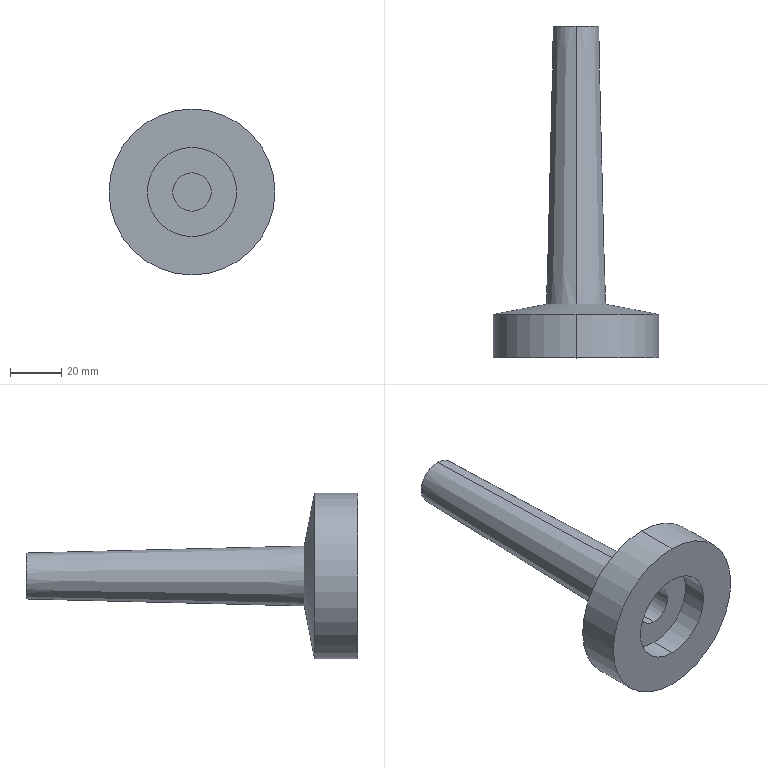Part | SolidWorks | features ICE 2, Revolution 1 | 1 solid | 14 faces | box 65 x 130 x 65 mm | volume 88701 mm3 | cylinder 6 | cone 4 | plane 4 | commonest cylinder face diameters 15 x2 35 x2 65 x2
STEP:
#1=CARTESIAN_POINT('',(0.,20.,7.5));
#2=VERTEX_POINT('',#1);
#3=CARTESIAN_POINT('',(0.,20.,-7.5));
#4=VERTEX_POINT('',#3);
#5=CARTESIAN_POINT('',(0.,20.,0.));
#6=DIRECTION('',(0.,-1.,0.));
#7=DIRECTION('',(0.,0.,-1.));
#8=AXIS2_PLACEMENT_3D('',#5,#6,#7);
#9=CIRCLE('',#8,7.5);
#10=EDGE_CURVE('',#2,#4,#9,.T.);
#11=ORIENTED_EDGE('',*,*,#10,.F.);
#12=CARTESIAN_POINT('',(0.,10.,7.5));
#13=VERTEX_POINT('',#12);
#14=CARTESIAN_POINT('',(0.,20.,7.5));
#15=DIRECTION('',(0.,-1.,0.));
#16=VECTOR('',#15,1000.);
#17=LINE('',#14,#16);
#18=EDGE_CURVE('',#2,#13,#17,.T.);
#19=ORIENTED_EDGE('',*,*,#18,.T.);
#20=CARTESIAN_POINT('',(0.,10.,-7.5));
#21=VERTEX_POINT('',#20);
#22=CARTESIAN_POINT('',(0.,10.,0.));
#23=DIRECTION('',(0.,-1.,0.));
#24=DIRECTION('',(0.,0.,-1.));
#25=AXIS2_PLACEMENT_3D('',#22,#23,#24);
#26=CIRCLE('',#25,7.5);
#27=EDGE_CURVE('',#13,#21,#26,.T.);
#28=ORIENTED_EDGE('',*,*,#27,.T.);
#29=CARTESIAN_POINT('',(0.,20.,-7.5));
#30=DIRECTION('',(0.,-1.,0.));
#31=VECTOR('',#30,1000.);
#32=LINE('',#29,#31);
#33=EDGE_CURVE('',#4,#21,#32,.T.);
#34=ORIENTED_EDGE('',*,*,#33,.F.);
#35=EDGE_LOOP('',(#11,#19,#28,#34));
#36=FACE_OUTER_BOUND('',#35,.T.);
#37=CARTESIAN_POINT('',(0.,20.,0.));
#38=DIRECTION('',(0.,-1.,0.));
#39=DIRECTION('',(0.,0.,-1.));
#40=AXIS2_PLACEMENT_3D('',#37,#38,#39);
#41=CYLINDRICAL_SURFACE('',#40,7.5);
#42=ADVANCED_FACE('',(#36),#41,.F.);
#43=CARTESIAN_POINT('',(0.,10.,17.5));
#44=VERTEX_POINT('',#43);
#45=CARTESIAN_POINT('',(0.,10.,-17.5));
#46=VERTEX_POINT('',#45);
#47=CARTESIAN_POINT('',(0.,10.,0.));
#48=DIRECTION('',(0.,-1.,0.));
#49=DIRECTION('',(0.,0.,-1.));
#50=AXIS2_PLACEMENT_3D('',#47,#48,#49);
#51=CIRCLE('',#50,17.5);
#52=EDGE_CURVE('',#44,#46,#51,.T.);
#53=ORIENTED_EDGE('',*,*,#52,.F.);
#54=CARTESIAN_POINT('',(0.,0.,17.5));
#55=VERTEX_POINT('',#54);
#56=CARTESIAN_POINT('',(0.,10.,17.5));
#57=DIRECTION('',(0.,-1.,0.));
#58=VECTOR('',#57,1000.);
#59=LINE('',#56,#58);
#60=EDGE_CURVE('',#44,#55,#59,.T.);
#61=ORIENTED_EDGE('',*,*,#60,.T.);
#62=CARTESIAN_POINT('',(0.,0.,-17.5));
#63=VERTEX_POINT('',#62);
#64=CARTESIAN_POINT('',(0.,0.,0.));
#65=DIRECTION('',(0.,-1.,0.));
#66=DIRECTION('',(0.,0.,-1.));
#67=AXIS2_PLACEMENT_3D('',#64,#65,#66);
#68=CIRCLE('',#67,17.5);
#69=EDGE_CURVE('',#55,#63,#68,.T.);
#70=ORIENTED_EDGE('',*,*,#69,.T.);
#71=CARTESIAN_POINT('',(0.,10.,-17.5));
#72=DIRECTION('',(0.,-1.,0.));
#73=VECTOR('',#72,1000.);
#74=LINE('',#71,#73);
#75=EDGE_CURVE('',#46,#63,#74,.T.);
#76=ORIENTED_EDGE('',*,*,#75,.F.);
#77=EDGE_LOOP('',(#53,#61,#70,#76));
#78=FACE_OUTER_BOUND('',#77,.T.);
#79=CARTESIAN_POINT('',(0.,10.,0.));
#80=DIRECTION('',(0.,-1.,0.));
#81=DIRECTION('',(0.,0.,-1.));
#82=AXIS2_PLACEMENT_3D('',#79,#80,#81);
#83=CYLINDRICAL_SURFACE('',#82,17.5);
#84=ADVANCED_FACE('',(#78),#83,.F.);
#85=CARTESIAN_POINT('',(0.,17.,-32.5));
#86=VERTEX_POINT('',#85);
#87=CARTESIAN_POINT('',(0.,17.,32.5));
#88=VERTEX_POINT('',#87);
#89=CARTESIAN_POINT('',(0.,17.,0.));
#90=DIRECTION('',(0.,-1.,0.));
#91=DIRECTION('',(0.,0.,-1.));
#92=AXIS2_PLACEMENT_3D('',#89,#90,#91);
#93=CIRCLE('',#92,32.5);
#94=EDGE_CURVE('',#86,#88,#93,.T.);
#95=ORIENTED_EDGE('',*,*,#94,.T.);
#96=CARTESIAN_POINT('',(0.,0.,32.5));
#97=VERTEX_POINT('',#96);
#98=CARTESIAN_POINT('',(0.,0.,32.5));
#99=DIRECTION('',(0.,-1.,0.));
#100=VECTOR('',#99,1000.);
#101=LINE('',#98,#100);
#102=EDGE_CURVE('',#88,#97,#101,.T.);
#103=ORIENTED_EDGE('',*,*,#102,.T.);
#104=CARTESIAN_POINT('',(0.,0.,-32.5));
#105=VERTEX_POINT('',#104);
#106=CARTESIAN_POINT('',(0.,0.,0.));
#107=DIRECTION('',(0.,-1.,0.));
#108=DIRECTION('',(0.,0.,-1.));
#109=AXIS2_PLACEMENT_3D('',#106,#107,#108);
#110=CIRCLE('',#109,32.5);
#111=EDGE_CURVE('',#105,#97,#110,.T.);
#112=ORIENTED_EDGE('',*,*,#111,.F.);
#113=CARTESIAN_POINT('',(0.,0.,-32.5));
#114=DIRECTION('',(0.,-1.,0.));
#115=VECTOR('',#114,1000.);
#116=LINE('',#113,#115);
#117=EDGE_CURVE('',#86,#105,#116,.T.);
#118=ORIENTED_EDGE('',*,*,#117,.F.);
#119=EDGE_LOOP('',(#95,#103,#112,#118));
#120=FACE_OUTER_BOUND('',#119,.T.);
#121=CARTESIAN_POINT('',(0.,0.,0.));
#122=DIRECTION('',(0.,-1.,0.));
#123=DIRECTION('',(0.,0.,-1.));
#124=AXIS2_PLACEMENT_3D('',#121,#122,#123);
#125=CYLINDRICAL_SURFACE('',#124,32.5);
#126=ADVANCED_FACE('',(#120),#125,.T.);
#127=CARTESIAN_POINT('',(0.,21.,-11.75));
#128=VERTEX_POINT('',#127);
#129=CARTESIAN_POINT('',(0.,21.,11.75));
#130=VERTEX_POINT('',#129);
#131=CARTESIAN_POINT('',(0.,21.,0.));
#132=DIRECTION('',(0.,-1.,0.));
#133=DIRECTION('',(0.,0.,-1.));
#134=AXIS2_PLACEMENT_3D('',#131,#132,#133);
#135=CIRCLE('',#134,11.75);
#136=EDGE_CURVE('',#128,#130,#135,.T.);
#137=ORIENTED_EDGE('',*,*,#136,.T.);
#138=CARTESIAN_POINT('',(0.,17.,32.5));
#139=DIRECTION('',(0.,-0.1893,0.9819));
#140=VECTOR('',#139,1000.);
#141=LINE('',#138,#140);
#142=EDGE_CURVE('',#130,#88,#141,.T.);
#143=ORIENTED_EDGE('',*,*,#142,.T.);
#144=ORIENTED_EDGE('',*,*,#94,.F.);
#145=CARTESIAN_POINT('',(0.,17.,-32.5));
#146=DIRECTION('',(0.,-0.1893,-0.9819));
#147=VECTOR('',#146,1000.);
#148=LINE('',#145,#147);
#149=EDGE_CURVE('',#128,#86,#148,.T.);
#150=ORIENTED_EDGE('',*,*,#149,.F.);
#151=EDGE_LOOP('',(#137,#143,#144,#150));
#152=FACE_OUTER_BOUND('',#151,.T.);
#153=CARTESIAN_POINT('',(0.,17.,0.));
#154=DIRECTION('',(0.,-1.,0.));
#155=DIRECTION('',(0.,0.,-1.));
#156=AXIS2_PLACEMENT_3D('',#153,#154,#155);
#157=CONICAL_SURFACE('',#156,32.5,1.38);
#158=ADVANCED_FACE('',(#152),#157,.T.);
#159=CARTESIAN_POINT('',(0.,130.,-9.));
#160=VERTEX_POINT('',#159);
#161=CARTESIAN_POINT('',(0.,130.,9.));
#162=VERTEX_POINT('',#161);
#163=CARTESIAN_POINT('',(0.,130.,0.));
#164=DIRECTION('',(0.,-1.,0.));
#165=DIRECTION('',(0.,0.,-1.));
#166=AXIS2_PLACEMENT_3D('',#163,#164,#165);
#167=CIRCLE('',#166,9.);
#168=EDGE_CURVE('',#160,#162,#167,.T.);
#169=ORIENTED_EDGE('',*,*,#168,.T.);
#170=CARTESIAN_POINT('',(0.,21.,11.75));
#171=DIRECTION('',(0.,-0.9997,0.02522));
#172=VECTOR('',#171,1000.);
#173=LINE('',#170,#172);
#174=EDGE_CURVE('',#162,#130,#173,.T.);
#175=ORIENTED_EDGE('',*,*,#174,.T.);
#176=ORIENTED_EDGE('',*,*,#136,.F.);
#177=CARTESIAN_POINT('',(0.,21.,-11.75));
#178=DIRECTION('',(0.,-0.9997,-0.02522));
#179=VECTOR('',#178,1000.);
#180=LINE('',#177,#179);
#181=EDGE_CURVE('',#160,#128,#180,.T.);
#182=ORIENTED_EDGE('',*,*,#181,.F.);
#183=EDGE_LOOP('',(#169,#175,#176,#182));
#184=FACE_OUTER_BOUND('',#183,.T.);
#185=CARTESIAN_POINT('',(0.,21.,0.));
#186=DIRECTION('',(0.,-1.,0.));
#187=DIRECTION('',(0.,0.,-1.));
#188=AXIS2_PLACEMENT_3D('',#185,#186,#187);
#189=CONICAL_SURFACE('',#188,11.75,0.02522);
#190=ADVANCED_FACE('',(#184),#189,.T.);
#191=CARTESIAN_POINT('',(0.,0.,0.));
#192=DIRECTION('',(0.,-1.,0.));
#193=DIRECTION('',(0.,0.,-1.));
#194=AXIS2_PLACEMENT_3D('',#191,#192,#193);
#195=CIRCLE('',#194,17.5);
#196=EDGE_CURVE('',#63,#55,#195,.T.);
#197=ORIENTED_EDGE('',*,*,#196,.F.);
#198=ORIENTED_EDGE('',*,*,#69,.F.);
#199=EDGE_LOOP('',(#197,#198));
#200=FACE_BOUND('',#199,.T.);
#201=ORIENTED_EDGE('',*,*,#111,.T.);
#202=CARTESIAN_POINT('',(0.,0.,0.));
#203=DIRECTION('',(0.,-1.,0.));
#204=DIRECTION('',(0.,0.,-1.));
#205=AXIS2_PLACEMENT_3D('',#202,#203,#204);
#206=CIRCLE('',#205,32.5);
#207=EDGE_CURVE('',#97,#105,#206,.T.);
#208=ORIENTED_EDGE('',*,*,#207,.T.);
#209=EDGE_LOOP('',(#201,#208));
#210=FACE_OUTER_BOUND('',#209,.T.);
#211=CARTESIAN_POINT('',(0.,0.,0.));
#212=DIRECTION('',(0.,-1.,0.));
#213=DIRECTION('',(0.,0.,-1.));
#214=AXIS2_PLACEMENT_3D('',#211,#212,#213);
#215=PLANE('',#214);
#216=ADVANCED_FACE('',(#200,#210),#215,.T.);
#217=ORIENTED_EDGE('',*,*,#168,.F.);
#218=CARTESIAN_POINT('',(0.,130.,0.));
#219=DIRECTION('',(0.,-1.,0.));
#220=DIRECTION('',(0.,0.,-1.));
#221=AXIS2_PLACEMENT_3D('',#218,#219,#220);
#222=CIRCLE('',#221,9.);
#223=EDGE_CURVE('',#162,#160,#222,.T.);
#224=ORIENTED_EDGE('',*,*,#223,.F.);
#225=EDGE_LOOP('',(#217,#224));
#226=FACE_OUTER_BOUND('',#225,.T.);
#227=CARTESIAN_POINT('',(0.,130.,0.));
#228=DIRECTION('',(0.,1.,0.));
#229=DIRECTION('',(0.,0.,1.));
#230=AXIS2_PLACEMENT_3D('',#227,#228,#229);
#231=PLANE('',#230);
#232=ADVANCED_FACE('',(#226),#231,.T.);
#233=ORIENTED_EDGE('',*,*,#174,.F.);
#234=ORIENTED_EDGE('',*,*,#223,.T.);
#235=ORIENTED_EDGE('',*,*,#181,.T.);
#236=CARTESIAN_POINT('',(0.,21.,0.));
#237=DIRECTION('',(0.,-1.,0.));
#238=DIRECTION('',(0.,0.,-1.));
#239=AXIS2_PLACEMENT_3D('',#236,#237,#238);
#240=CIRCLE('',#239,11.75);
#241=EDGE_CURVE('',#130,#128,#240,.T.);
#242=ORIENTED_EDGE('',*,*,#241,.F.);
#243=EDGE_LOOP('',(#233,#234,#235,#242));
#244=FACE_OUTER_BOUND('',#243,.T.);
#245=CARTESIAN_POINT('',(0.,21.,0.));
#246=DIRECTION('',(0.,-1.,0.));
#247=DIRECTION('',(0.,0.,-1.));
#248=AXIS2_PLACEMENT_3D('',#245,#246,#247);
#249=CONICAL_SURFACE('',#248,11.75,0.02522);
#250=ADVANCED_FACE('',(#244),#249,.T.);
#251=ORIENTED_EDGE('',*,*,#142,.F.);
#252=ORIENTED_EDGE('',*,*,#241,.T.);
#253=ORIENTED_EDGE('',*,*,#149,.T.);
#254=CARTESIAN_POINT('',(0.,17.,0.));
#255=DIRECTION('',(0.,-1.,0.));
#256=DIRECTION('',(0.,0.,-1.));
#257=AXIS2_PLACEMENT_3D('',#254,#255,#256);
#258=CIRCLE('',#257,32.5);
#259=EDGE_CURVE('',#88,#86,#258,.T.);
#260=ORIENTED_EDGE('',*,*,#259,.F.);
#261=EDGE_LOOP('',(#251,#252,#253,#260));
#262=FACE_OUTER_BOUND('',#261,.T.);
#263=CARTESIAN_POINT('',(0.,17.,0.));
#264=DIRECTION('',(0.,-1.,0.));
#265=DIRECTION('',(0.,0.,-1.));
#266=AXIS2_PLACEMENT_3D('',#263,#264,#265);
#267=CONICAL_SURFACE('',#266,32.5,1.38);
#268=ADVANCED_FACE('',(#262),#267,.T.);
#269=ORIENTED_EDGE('',*,*,#102,.F.);
#270=ORIENTED_EDGE('',*,*,#259,.T.);
#271=ORIENTED_EDGE('',*,*,#117,.T.);
#272=ORIENTED_EDGE('',*,*,#207,.F.);
#273=EDGE_LOOP('',(#269,#270,#271,#272));
#274=FACE_OUTER_BOUND('',#273,.T.);
#275=CARTESIAN_POINT('',(0.,0.,0.));
#276=DIRECTION('',(0.,-1.,0.));
#277=DIRECTION('',(0.,0.,-1.));
#278=AXIS2_PLACEMENT_3D('',#275,#276,#277);
#279=CYLINDRICAL_SURFACE('',#278,32.5);
#280=ADVANCED_FACE('',(#274),#279,.T.);
#281=ORIENTED_EDGE('',*,*,#60,.F.);
#282=CARTESIAN_POINT('',(0.,10.,0.));
#283=DIRECTION('',(0.,-1.,0.));
#284=DIRECTION('',(0.,0.,-1.));
#285=AXIS2_PLACEMENT_3D('',#282,#283,#284);
#286=CIRCLE('',#285,17.5);
#287=EDGE_CURVE('',#46,#44,#286,.T.);
#288=ORIENTED_EDGE('',*,*,#287,.F.);
#289=ORIENTED_EDGE('',*,*,#75,.T.);
#290=ORIENTED_EDGE('',*,*,#196,.T.);
#291=EDGE_LOOP('',(#281,#288,#289,#290));
#292=FACE_OUTER_BOUND('',#291,.T.);
#293=CARTESIAN_POINT('',(0.,10.,0.));
#294=DIRECTION('',(0.,-1.,0.));
#295=DIRECTION('',(0.,0.,-1.));
#296=AXIS2_PLACEMENT_3D('',#293,#294,#295);
#297=CYLINDRICAL_SURFACE('',#296,17.5);
#298=ADVANCED_FACE('',(#292),#297,.F.);
#299=CARTESIAN_POINT('',(0.,10.,0.));
#300=DIRECTION('',(0.,-1.,0.));
#301=DIRECTION('',(0.,0.,-1.));
#302=AXIS2_PLACEMENT_3D('',#299,#300,#301);
#303=CIRCLE('',#302,7.5);
#304=EDGE_CURVE('',#21,#13,#303,.T.);
#305=ORIENTED_EDGE('',*,*,#304,.F.);
#306=ORIENTED_EDGE('',*,*,#27,.F.);
#307=EDGE_LOOP('',(#305,#306));
#308=FACE_BOUND('',#307,.T.);
#309=ORIENTED_EDGE('',*,*,#287,.T.);
#310=ORIENTED_EDGE('',*,*,#52,.T.);
#311=EDGE_LOOP('',(#309,#310));
#312=FACE_OUTER_BOUND('',#311,.T.);
#313=CARTESIAN_POINT('',(0.,10.,0.));
#314=DIRECTION('',(0.,-1.,0.));
#315=DIRECTION('',(0.,0.,-1.));
#316=AXIS2_PLACEMENT_3D('',#313,#314,#315);
#317=PLANE('',#316);
#318=ADVANCED_FACE('',(#308,#312),#317,.T.);
#319=ORIENTED_EDGE('',*,*,#18,.F.);
#320=CARTESIAN_POINT('',(0.,20.,0.));
#321=DIRECTION('',(0.,-1.,0.));
#322=DIRECTION('',(0.,0.,-1.));
#323=AXIS2_PLACEMENT_3D('',#320,#321,#322);
#324=CIRCLE('',#323,7.5);
#325=EDGE_CURVE('',#4,#2,#324,.T.);
#326=ORIENTED_EDGE('',*,*,#325,.F.);
#327=ORIENTED_EDGE('',*,*,#33,.T.);
#328=ORIENTED_EDGE('',*,*,#304,.T.);
#329=EDGE_LOOP('',(#319,#326,#327,#328));
#330=FACE_OUTER_BOUND('',#329,.T.);
#331=CARTESIAN_POINT('',(0.,20.,0.));
#332=DIRECTION('',(0.,-1.,0.));
#333=DIRECTION('',(0.,0.,-1.));
#334=AXIS2_PLACEMENT_3D('',#331,#332,#333);
#335=CYLINDRICAL_SURFACE('',#334,7.5);
#336=ADVANCED_FACE('',(#330),#335,.F.);
#337=ORIENTED_EDGE('',*,*,#325,.T.);
#338=ORIENTED_EDGE('',*,*,#10,.T.);
#339=EDGE_LOOP('',(#337,#338));
#340=FACE_OUTER_BOUND('',#339,.T.);
#341=CARTESIAN_POINT('',(0.,20.,0.));
#342=DIRECTION('',(0.,-1.,0.));
#343=DIRECTION('',(0.,0.,-1.));
#344=AXIS2_PLACEMENT_3D('',#341,#342,#343);
#345=PLANE('',#344);
#346=ADVANCED_FACE('',(#340),#345,.T.);
#347=CLOSED_SHELL('',(#42,#84,#126,#158,#190,#216,#232,#250,#268,#280,#298,#318,#336,#346));
#348=MANIFOLD_SOLID_BREP('',#347);
#349=CARTESIAN_POINT('',(0.,0.,0.));
#350=DIRECTION('',(0.,0.,1.));
#351=DIRECTION('',(1.,0.,0.));
#352=AXIS2_PLACEMENT_3D('',#349,#350,#351);
#353=(LENGTH_UNIT()NAMED_UNIT(*)SI_UNIT(.MILLI.,.METRE.));
#354=UNCERTAINTY_MEASURE_WITH_UNIT(LENGTH_MEASURE(0.00001),#353,'','');
#355=(NAMED_UNIT(*)PLANE_ANGLE_UNIT()SI_UNIT($,.RADIAN.));
#356=(NAMED_UNIT(*)SI_UNIT($,.STERADIAN.)SOLID_ANGLE_UNIT());
#357=(GEOMETRIC_REPRESENTATION_CONTEXT(3)GLOBAL_UNCERTAINTY_ASSIGNED_CONTEXT((#354))GLOBAL_UNIT_ASSIGNED_CONTEXT((#353,#355,#356))REPRESENTATION_CONTEXT('',''));
#358=ADVANCED_BREP_SHAPE_REPRESENTATION('',(#348,#352),#357);